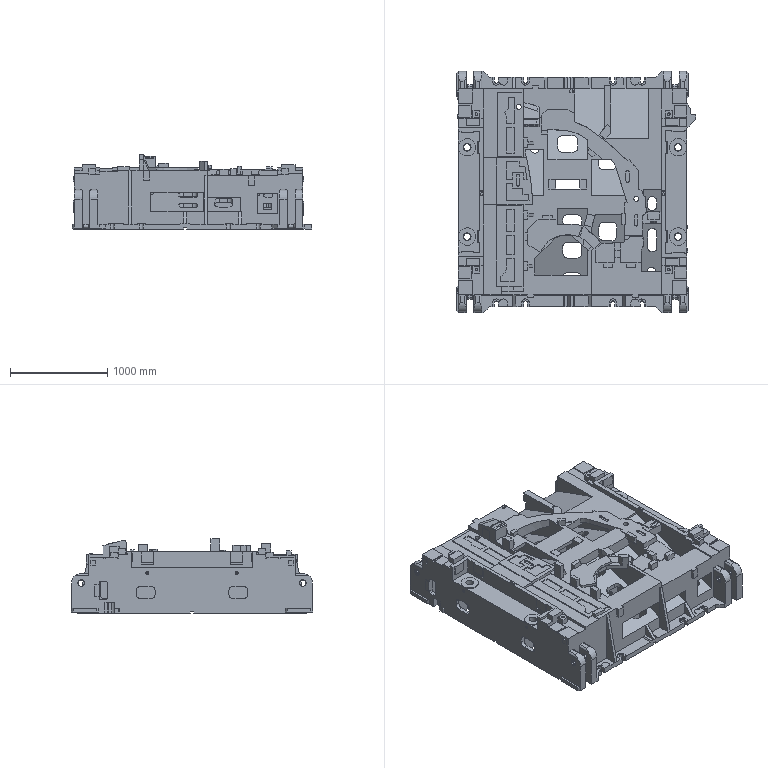Part | NX | features solid 2 | 1 solid | 2145 faces | box 2460 x 2480 x 765 mm | volume 964801737 mm3 | plane 1592 | cylinder 438 | spline 107 | torus 8 | commonest cylinder face diameters 80 x180 68 x48 40 x44 100 x40 60 x38 30 x22